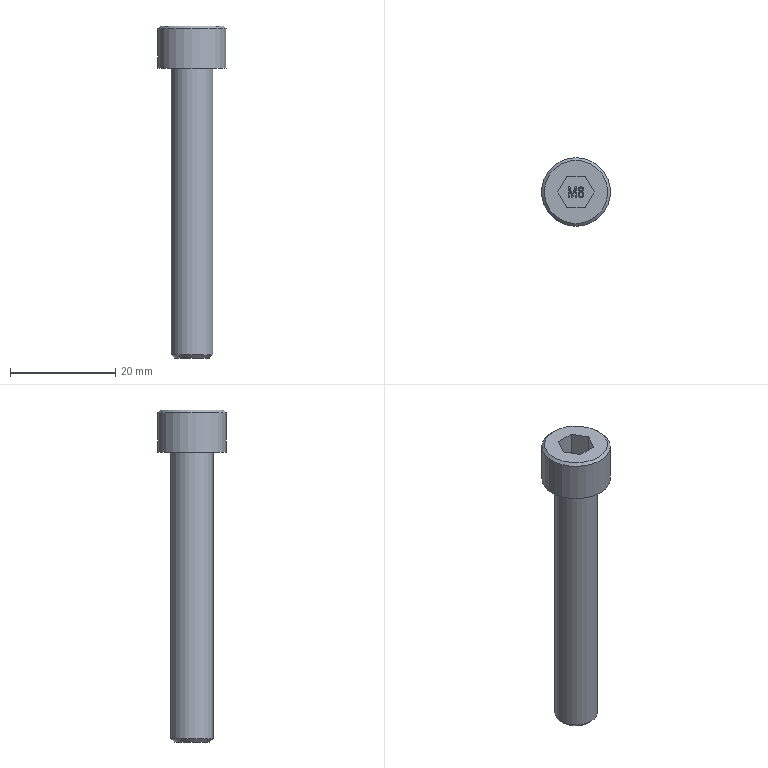Part | STEP file | EM10805500 | 1 solid | 38 faces | box 13 x 13 x 63 mm | volume 3662 mm3 | plane 25 | other 9 | cylinder 2 | cone 2 | commonest cylinder face diameters 8 x1 13 x1